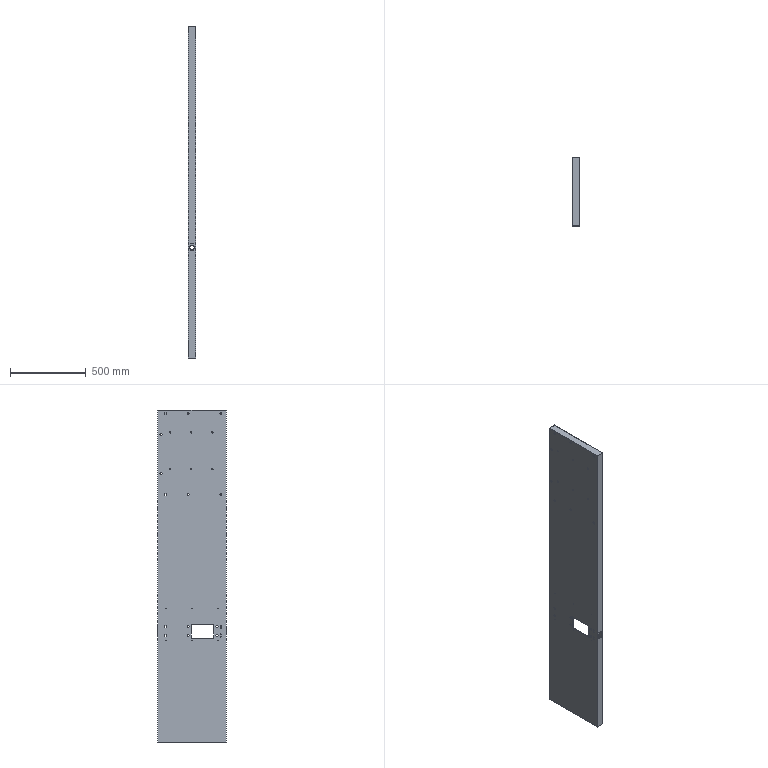Part | SolidWorks | features BaseBody 1 | 1 solid | 175 faces | box 50 x 450 x 2190 mm | volume 3387265 mm3 | plane 113 | cylinder 54 | cone 8 | commonest cylinder face diameters 5.5 x16 4.4 x12 8.5 x12 11 x6 10.6 x4 30 x2